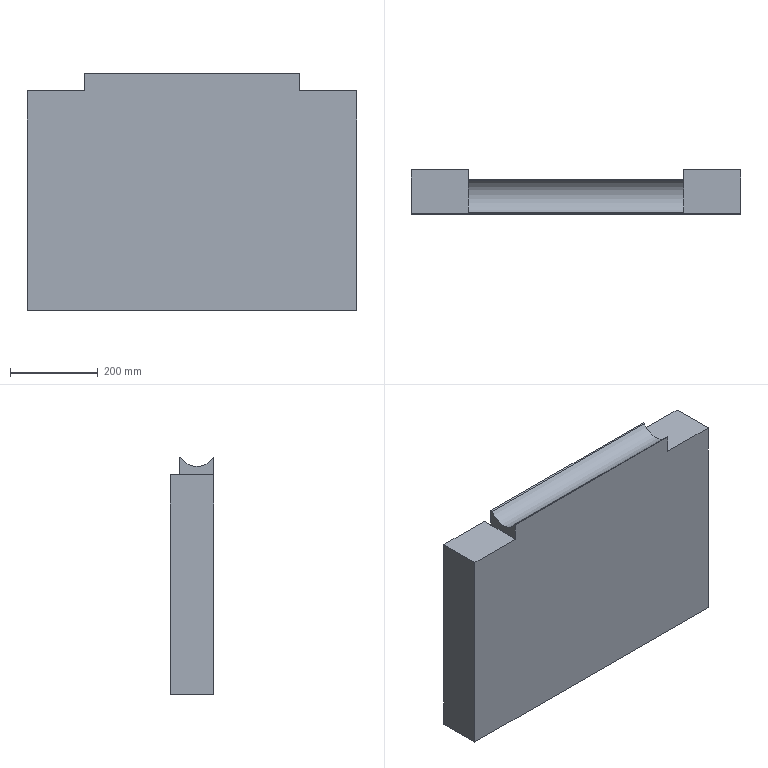Part | STEP file | 1 solid | 16 faces | box 750 x 100 x 540 mm | volume 33368808 mm3 | plane 15 | cylinder 1 | commonest cylinder face diameters 85 x1
STEP:
#1=CARTESIAN_POINT('',(0.,0.,0.));
#2=DIRECTION('',(0.,0.,1.));
#3=DIRECTION('',(1.,0.,0.));
#4=AXIS2_PLACEMENT_3D('',#1,#2,#3);
#5=CARTESIAN_POINT('',(375.,-50.,500.));
#6=VERTEX_POINT('',#5);
#7=CARTESIAN_POINT('',(375.,-50.,0.));
#8=VERTEX_POINT('',#7);
#9=CARTESIAN_POINT('',(375.,-50.,500.));
#10=DIRECTION('',(0.,0.,-1.));
#11=VECTOR('',#10,1.);
#12=LINE('',#9,#11);
#13=CARTESIAN_POINT('',(-375.,-50.,500.));
#14=DIRECTION('',(0.,1.,0.));
#15=DIRECTION('',(0.,0.,1.));
#16=AXIS2_PLACEMENT_3D('',#13,#14,#15);
#17=PLANE('',#16);
#18=CARTESIAN_POINT('',(0.,750.));
#19=DIRECTION('',(-1.,0.));
#20=VECTOR('',#19,1.);
#21=LINE('',#18,#20);
#22=(GEOMETRIC_REPRESENTATION_CONTEXT(2)PARAMETRIC_REPRESENTATION_CONTEXT()REPRESENTATION_CONTEXT('',''));
#23=DEFINITIONAL_REPRESENTATION('',(#21),#22);
#24=PCURVE('',#17,#23);
#25=CARTESIAN_POINT('',(375.,50.,500.));
#26=DIRECTION('',(-1.,0.,0.));
#27=DIRECTION('',(0.,0.,1.));
#28=AXIS2_PLACEMENT_3D('',#25,#26,#27);
#29=PLANE('',#28);
#30=CARTESIAN_POINT('',(0.,-100.));
#31=DIRECTION('',(-1.,0.));
#32=VECTOR('',#31,1.);
#33=LINE('',#30,#32);
#34=(GEOMETRIC_REPRESENTATION_CONTEXT(2)PARAMETRIC_REPRESENTATION_CONTEXT()REPRESENTATION_CONTEXT('',''));
#35=DEFINITIONAL_REPRESENTATION('',(#33),#34);
#36=PCURVE('',#29,#35);
#37=SURFACE_CURVE('',#12,(#24,#36),.PCURVE_S1.);
#38=EDGE_CURVE('',#6,#8,#37,.T.);
#39=ORIENTED_EDGE('',*,*,#38,.F.);
#40=CARTESIAN_POINT('',(245.,-50.,500.));
#41=VERTEX_POINT('',#40);
#42=CARTESIAN_POINT('',(-375.,-50.,500.));
#43=DIRECTION('',(1.,0.,0.));
#44=VECTOR('',#43,1.);
#45=LINE('',#42,#44);
#46=CARTESIAN_POINT('',(0.,0.));
#47=DIRECTION('',(0.,1.));
#48=VECTOR('',#47,1.);
#49=LINE('',#46,#48);
#50=(GEOMETRIC_REPRESENTATION_CONTEXT(2)PARAMETRIC_REPRESENTATION_CONTEXT()REPRESENTATION_CONTEXT('',''));
#51=DEFINITIONAL_REPRESENTATION('',(#49),#50);
#52=PCURVE('',#17,#51);
#53=CARTESIAN_POINT('',(0.,0.,500.));
#54=DIRECTION('',(0.,0.,1.));
#55=DIRECTION('',(1.,0.,0.));
#56=AXIS2_PLACEMENT_3D('',#53,#54,#55);
#57=PLANE('',#56);
#58=CARTESIAN_POINT('',(-375.,-50.));
#59=DIRECTION('',(1.,0.));
#60=VECTOR('',#59,1.);
#61=LINE('',#58,#60);
#62=(GEOMETRIC_REPRESENTATION_CONTEXT(2)PARAMETRIC_REPRESENTATION_CONTEXT()REPRESENTATION_CONTEXT('',''));
#63=DEFINITIONAL_REPRESENTATION('',(#61),#62);
#64=PCURVE('',#57,#63);
#65=SURFACE_CURVE('',#45,(#52,#64),.PCURVE_S1.);
#66=EDGE_CURVE('',#41,#6,#65,.T.);
#67=ORIENTED_EDGE('',*,*,#66,.F.);
#68=CARTESIAN_POINT('',(245.,-50.,540.));
#69=VERTEX_POINT('',#68);
#70=CARTESIAN_POINT('',(245.,-50.,500.));
#71=DIRECTION('',(0.,0.,-1.));
#72=VECTOR('',#71,1.);
#73=LINE('',#70,#72);
#74=CARTESIAN_POINT('',(0.,620.));
#75=DIRECTION('',(-1.,0.));
#76=VECTOR('',#75,1.);
#77=LINE('',#74,#76);
#78=(GEOMETRIC_REPRESENTATION_CONTEXT(2)PARAMETRIC_REPRESENTATION_CONTEXT()REPRESENTATION_CONTEXT('',''));
#79=DEFINITIONAL_REPRESENTATION('',(#77),#78);
#80=PCURVE('',#17,#79);
#81=CARTESIAN_POINT('',(245.,29.,540.));
#82=DIRECTION('',(-1.,0.,0.));
#83=DIRECTION('',(0.,0.,1.));
#84=AXIS2_PLACEMENT_3D('',#81,#82,#83);
#85=PLANE('',#84);
#86=CARTESIAN_POINT('',(-40.,-79.));
#87=DIRECTION('',(-1.,0.));
#88=VECTOR('',#87,1.);
#89=LINE('',#86,#88);
#90=(GEOMETRIC_REPRESENTATION_CONTEXT(2)PARAMETRIC_REPRESENTATION_CONTEXT()REPRESENTATION_CONTEXT('',''));
#91=DEFINITIONAL_REPRESENTATION('',(#89),#90);
#92=PCURVE('',#85,#91);
#93=SURFACE_CURVE('',#73,(#80,#92),.PCURVE_S1.);
#94=EDGE_CURVE('',#69,#41,#93,.T.);
#95=ORIENTED_EDGE('',*,*,#94,.F.);
#96=CARTESIAN_POINT('',(-245.,-50.,540.));
#97=VERTEX_POINT('',#96);
#98=CARTESIAN_POINT('',(-375.,-50.,540.));
#99=DIRECTION('',(1.,0.,0.));
#100=VECTOR('',#99,1.);
#101=LINE('',#98,#100);
#102=CARTESIAN_POINT('',(40.,0.));
#103=DIRECTION('',(0.,1.));
#104=VECTOR('',#103,1.);
#105=LINE('',#102,#104);
#106=(GEOMETRIC_REPRESENTATION_CONTEXT(2)PARAMETRIC_REPRESENTATION_CONTEXT()REPRESENTATION_CONTEXT('',''));
#107=DEFINITIONAL_REPRESENTATION('',(#105),#106);
#108=PCURVE('',#17,#107);
#109=CARTESIAN_POINT('',(0.,0.,540.));
#110=DIRECTION('',(0.,0.,1.));
#111=DIRECTION('',(1.,0.,0.));
#112=AXIS2_PLACEMENT_3D('',#109,#110,#111);
#113=PLANE('',#112);
#114=CARTESIAN_POINT('',(-375.,-50.));
#115=DIRECTION('',(1.,0.));
#116=VECTOR('',#115,1.);
#117=LINE('',#114,#116);
#118=(GEOMETRIC_REPRESENTATION_CONTEXT(2)PARAMETRIC_REPRESENTATION_CONTEXT()REPRESENTATION_CONTEXT('',''));
#119=DEFINITIONAL_REPRESENTATION('',(#117),#118);
#120=PCURVE('',#113,#119);
#121=SURFACE_CURVE('',#101,(#108,#120),.PCURVE_S1.);
#122=EDGE_CURVE('',#97,#69,#121,.T.);
#123=ORIENTED_EDGE('',*,*,#122,.F.);
#124=CARTESIAN_POINT('',(-245.,-50.,500.));
#125=VERTEX_POINT('',#124);
#126=CARTESIAN_POINT('',(-245.,-50.,500.));
#127=DIRECTION('',(0.,0.,1.));
#128=VECTOR('',#127,1.);
#129=LINE('',#126,#128);
#130=CARTESIAN_POINT('',(0.,130.));
#131=DIRECTION('',(1.,0.));
#132=VECTOR('',#131,1.);
#133=LINE('',#130,#132);
#134=(GEOMETRIC_REPRESENTATION_CONTEXT(2)PARAMETRIC_REPRESENTATION_CONTEXT()REPRESENTATION_CONTEXT('',''));
#135=DEFINITIONAL_REPRESENTATION('',(#133),#134);
#136=PCURVE('',#17,#135);
#137=CARTESIAN_POINT('',(-245.,29.,540.));
#138=DIRECTION('',(1.,0.,0.));
#139=DIRECTION('',(0.,0.,-1.));
#140=AXIS2_PLACEMENT_3D('',#137,#138,#139);
#141=PLANE('',#140);
#142=CARTESIAN_POINT('',(40.,-79.));
#143=DIRECTION('',(-1.,0.));
#144=VECTOR('',#143,1.);
#145=LINE('',#142,#144);
#146=(GEOMETRIC_REPRESENTATION_CONTEXT(2)PARAMETRIC_REPRESENTATION_CONTEXT()REPRESENTATION_CONTEXT('',''));
#147=DEFINITIONAL_REPRESENTATION('',(#145),#146);
#148=PCURVE('',#141,#147);
#149=SURFACE_CURVE('',#129,(#136,#148),.PCURVE_S1.);
#150=EDGE_CURVE('',#125,#97,#149,.T.);
#151=ORIENTED_EDGE('',*,*,#150,.F.);
#152=CARTESIAN_POINT('',(-375.,-50.,500.));
#153=VERTEX_POINT('',#152);
#154=CARTESIAN_POINT('',(-375.,-50.,500.));
#155=DIRECTION('',(1.,0.,0.));
#156=VECTOR('',#155,1.);
#157=LINE('',#154,#156);
#158=CARTESIAN_POINT('',(0.,0.));
#159=DIRECTION('',(0.,1.));
#160=VECTOR('',#159,1.);
#161=LINE('',#158,#160);
#162=(GEOMETRIC_REPRESENTATION_CONTEXT(2)PARAMETRIC_REPRESENTATION_CONTEXT()REPRESENTATION_CONTEXT('',''));
#163=DEFINITIONAL_REPRESENTATION('',(#161),#162);
#164=PCURVE('',#17,#163);
#165=CARTESIAN_POINT('',(0.,0.,500.));
#166=DIRECTION('',(0.,0.,1.));
#167=DIRECTION('',(1.,0.,0.));
#168=AXIS2_PLACEMENT_3D('',#165,#166,#167);
#169=PLANE('',#168);
#170=CARTESIAN_POINT('',(-375.,-50.));
#171=DIRECTION('',(1.,0.));
#172=VECTOR('',#171,1.);
#173=LINE('',#170,#172);
#174=(GEOMETRIC_REPRESENTATION_CONTEXT(2)PARAMETRIC_REPRESENTATION_CONTEXT()REPRESENTATION_CONTEXT('',''));
#175=DEFINITIONAL_REPRESENTATION('',(#173),#174);
#176=PCURVE('',#169,#175);
#177=SURFACE_CURVE('',#157,(#164,#176),.PCURVE_S1.);
#178=EDGE_CURVE('',#153,#125,#177,.T.);
#179=ORIENTED_EDGE('',*,*,#178,.F.);
#180=CARTESIAN_POINT('',(-375.,-50.,0.));
#181=VERTEX_POINT('',#180);
#182=CARTESIAN_POINT('',(-375.,-50.,500.));
#183=DIRECTION('',(0.,0.,1.));
#184=VECTOR('',#183,1.);
#185=LINE('',#182,#184);
#186=CARTESIAN_POINT('',(0.,0.));
#187=DIRECTION('',(1.,0.));
#188=VECTOR('',#187,1.);
#189=LINE('',#186,#188);
#190=(GEOMETRIC_REPRESENTATION_CONTEXT(2)PARAMETRIC_REPRESENTATION_CONTEXT()REPRESENTATION_CONTEXT('',''));
#191=DEFINITIONAL_REPRESENTATION('',(#189),#190);
#192=PCURVE('',#17,#191);
#193=CARTESIAN_POINT('',(-375.,50.,500.));
#194=DIRECTION('',(1.,0.,0.));
#195=DIRECTION('',(0.,0.,-1.));
#196=AXIS2_PLACEMENT_3D('',#193,#194,#195);
#197=PLANE('',#196);
#198=CARTESIAN_POINT('',(0.,-100.));
#199=DIRECTION('',(-1.,0.));
#200=VECTOR('',#199,1.);
#201=LINE('',#198,#200);
#202=(GEOMETRIC_REPRESENTATION_CONTEXT(2)PARAMETRIC_REPRESENTATION_CONTEXT()REPRESENTATION_CONTEXT('',''));
#203=DEFINITIONAL_REPRESENTATION('',(#201),#202);
#204=PCURVE('',#197,#203);
#205=SURFACE_CURVE('',#185,(#192,#204),.PCURVE_S1.);
#206=EDGE_CURVE('',#181,#153,#205,.T.);
#207=ORIENTED_EDGE('',*,*,#206,.F.);
#208=CARTESIAN_POINT('',(-375.,-50.,0.));
#209=DIRECTION('',(-1.,0.,0.));
#210=VECTOR('',#209,1.);
#211=LINE('',#208,#210);
#212=CARTESIAN_POINT('',(-500.,0.));
#213=DIRECTION('',(0.,-1.));
#214=VECTOR('',#213,1.);
#215=LINE('',#212,#214);
#216=(GEOMETRIC_REPRESENTATION_CONTEXT(2)PARAMETRIC_REPRESENTATION_CONTEXT()REPRESENTATION_CONTEXT('',''));
#217=DEFINITIONAL_REPRESENTATION('',(#215),#216);
#218=PCURVE('',#17,#217);
#219=CARTESIAN_POINT('',(0.,0.,0.));
#220=DIRECTION('',(0.,0.,1.));
#221=DIRECTION('',(1.,0.,0.));
#222=AXIS2_PLACEMENT_3D('',#219,#220,#221);
#223=PLANE('',#222);
#224=CARTESIAN_POINT('',(-375.,-50.));
#225=DIRECTION('',(-1.,0.));
#226=VECTOR('',#225,1.);
#227=LINE('',#224,#226);
#228=(GEOMETRIC_REPRESENTATION_CONTEXT(2)PARAMETRIC_REPRESENTATION_CONTEXT()REPRESENTATION_CONTEXT('',''));
#229=DEFINITIONAL_REPRESENTATION('',(#227),#228);
#230=PCURVE('',#223,#229);
#231=SURFACE_CURVE('',#211,(#218,#230),.PCURVE_S1.);
#232=EDGE_CURVE('',#8,#181,#231,.T.);
#233=ORIENTED_EDGE('',*,*,#232,.F.);
#234=EDGE_LOOP('',(#39,#67,#95,#123,#151,#179,#207,#233));
#235=FACE_BOUND('',#234,.T.);
#236=ADVANCED_FACE('',(#235),#17,.F.);
#237=CARTESIAN_POINT('',(245.,50.,0.));
#238=VERTEX_POINT('',#237);
#239=CARTESIAN_POINT('',(245.,29.,0.));
#240=VERTEX_POINT('',#239);
#241=CARTESIAN_POINT('',(245.,0.,0.));
#242=DIRECTION('',(0.,-1.,0.));
#243=VECTOR('',#242,1.);
#244=LINE('',#241,#243);
#245=CARTESIAN_POINT('',(245.,0.));
#246=DIRECTION('',(0.,-1.));
#247=VECTOR('',#246,1.);
#248=LINE('',#245,#247);
#249=(GEOMETRIC_REPRESENTATION_CONTEXT(2)PARAMETRIC_REPRESENTATION_CONTEXT()REPRESENTATION_CONTEXT('',''));
#250=DEFINITIONAL_REPRESENTATION('',(#248),#249);
#251=PCURVE('',#223,#250);
#252=CARTESIAN_POINT('',(245.,71.,0.));
#253=DIRECTION('',(1.,0.,0.));
#254=DIRECTION('',(0.,0.,-1.));
#255=AXIS2_PLACEMENT_3D('',#252,#253,#254);
#256=PLANE('',#255);
#257=CARTESIAN_POINT('',(0.,-71.));
#258=DIRECTION('',(0.,-1.));
#259=VECTOR('',#258,1.);
#260=LINE('',#257,#259);
#261=(GEOMETRIC_REPRESENTATION_CONTEXT(2)PARAMETRIC_REPRESENTATION_CONTEXT()REPRESENTATION_CONTEXT('',''));
#262=DEFINITIONAL_REPRESENTATION('',(#260),#261);
#263=PCURVE('',#256,#262);
#264=SURFACE_CURVE('',#244,(#251,#263),.PCURVE_S1.);
#265=EDGE_CURVE('',#238,#240,#264,.T.);
#266=ORIENTED_EDGE('',*,*,#265,.F.);
#267=CARTESIAN_POINT('',(375.,50.,0.));
#268=VERTEX_POINT('',#267);
#269=CARTESIAN_POINT('',(0.,50.,0.));
#270=DIRECTION('',(-1.,0.,0.));
#271=VECTOR('',#270,1.);
#272=LINE('',#269,#271);
#273=CARTESIAN_POINT('',(0.,50.));
#274=DIRECTION('',(-1.,0.));
#275=VECTOR('',#274,1.);
#276=LINE('',#273,#275);
#277=(GEOMETRIC_REPRESENTATION_CONTEXT(2)PARAMETRIC_REPRESENTATION_CONTEXT()REPRESENTATION_CONTEXT('',''));
#278=DEFINITIONAL_REPRESENTATION('',(#276),#277);
#279=PCURVE('',#223,#278);
#280=CARTESIAN_POINT('',(-375.,50.,500.));
#281=DIRECTION('',(0.,-1.,0.));
#282=DIRECTION('',(0.,0.,-1.));
#283=AXIS2_PLACEMENT_3D('',#280,#281,#282);
#284=PLANE('',#283);
#285=CARTESIAN_POINT('',(500.,375.));
#286=DIRECTION('',(0.,-1.));
#287=VECTOR('',#286,1.);
#288=LINE('',#285,#287);
#289=(GEOMETRIC_REPRESENTATION_CONTEXT(2)PARAMETRIC_REPRESENTATION_CONTEXT()REPRESENTATION_CONTEXT('',''));
#290=DEFINITIONAL_REPRESENTATION('',(#288),#289);
#291=PCURVE('',#284,#290);
#292=SURFACE_CURVE('',#272,(#279,#291),.PCURVE_S1.);
#293=EDGE_CURVE('',#268,#238,#292,.T.);
#294=ORIENTED_EDGE('',*,*,#293,.F.);
#295=CARTESIAN_POINT('',(375.,0.,0.));
#296=DIRECTION('',(0.,1.,0.));
#297=VECTOR('',#296,1.);
#298=LINE('',#295,#297);
#299=CARTESIAN_POINT('',(375.,0.));
#300=DIRECTION('',(0.,1.));
#301=VECTOR('',#300,1.);
#302=LINE('',#299,#301);
#303=(GEOMETRIC_REPRESENTATION_CONTEXT(2)PARAMETRIC_REPRESENTATION_CONTEXT()REPRESENTATION_CONTEXT('',''));
#304=DEFINITIONAL_REPRESENTATION('',(#302),#303);
#305=PCURVE('',#223,#304);
#306=CARTESIAN_POINT('',(-500.,-50.));
#307=DIRECTION('',(0.,1.));
#308=VECTOR('',#307,1.);
#309=LINE('',#306,#308);
#310=(GEOMETRIC_REPRESENTATION_CONTEXT(2)PARAMETRIC_REPRESENTATION_CONTEXT()REPRESENTATION_CONTEXT('',''));
#311=DEFINITIONAL_REPRESENTATION('',(#309),#310);
#312=PCURVE('',#29,#311);
#313=SURFACE_CURVE('',#298,(#305,#312),.PCURVE_S1.);
#314=EDGE_CURVE('',#8,#268,#313,.T.);
#315=ORIENTED_EDGE('',*,*,#314,.F.);
#316=ORIENTED_EDGE('',*,*,#232,.T.);
#317=CARTESIAN_POINT('',(-375.,50.,0.));
#318=VERTEX_POINT('',#317);
#319=CARTESIAN_POINT('',(-375.,0.,0.));
#320=DIRECTION('',(0.,-1.,0.));
#321=VECTOR('',#320,1.);
#322=LINE('',#319,#321);
#323=CARTESIAN_POINT('',(-375.,0.));
#324=DIRECTION('',(0.,-1.));
#325=VECTOR('',#324,1.);
#326=LINE('',#323,#325);
#327=(GEOMETRIC_REPRESENTATION_CONTEXT(2)PARAMETRIC_REPRESENTATION_CONTEXT()REPRESENTATION_CONTEXT('',''));
#328=DEFINITIONAL_REPRESENTATION('',(#326),#327);
#329=PCURVE('',#223,#328);
#330=CARTESIAN_POINT('',(500.,-50.));
#331=DIRECTION('',(0.,-1.));
#332=VECTOR('',#331,1.);
#333=LINE('',#330,#332);
#334=(GEOMETRIC_REPRESENTATION_CONTEXT(2)PARAMETRIC_REPRESENTATION_CONTEXT()REPRESENTATION_CONTEXT('',''));
#335=DEFINITIONAL_REPRESENTATION('',(#333),#334);
#336=PCURVE('',#197,#335);
#337=SURFACE_CURVE('',#322,(#329,#336),.PCURVE_S1.);
#338=EDGE_CURVE('',#318,#181,#337,.T.);
#339=ORIENTED_EDGE('',*,*,#338,.F.);
#340=CARTESIAN_POINT('',(-245.,50.,0.));
#341=VERTEX_POINT('',#340);
#342=CARTESIAN_POINT('',(0.,50.,0.));
#343=DIRECTION('',(-1.,0.,0.));
#344=VECTOR('',#343,1.);
#345=LINE('',#342,#344);
#346=CARTESIAN_POINT('',(0.,50.));
#347=DIRECTION('',(-1.,0.));
#348=VECTOR('',#347,1.);
#349=LINE('',#346,#348);
#350=(GEOMETRIC_REPRESENTATION_CONTEXT(2)PARAMETRIC_REPRESENTATION_CONTEXT()REPRESENTATION_CONTEXT('',''));
#351=DEFINITIONAL_REPRESENTATION('',(#349),#350);
#352=PCURVE('',#223,#351);
#353=CARTESIAN_POINT('',(-375.,50.,500.));
#354=DIRECTION('',(0.,-1.,0.));
#355=DIRECTION('',(0.,0.,-1.));
#356=AXIS2_PLACEMENT_3D('',#353,#354,#355);
#357=PLANE('',#356);
#358=CARTESIAN_POINT('',(500.,375.));
#359=DIRECTION('',(0.,-1.));
#360=VECTOR('',#359,1.);
#361=LINE('',#358,#360);
#362=(GEOMETRIC_REPRESENTATION_CONTEXT(2)PARAMETRIC_REPRESENTATION_CONTEXT()REPRESENTATION_CONTEXT('',''));
#363=DEFINITIONAL_REPRESENTATION('',(#361),#362);
#364=PCURVE('',#357,#363);
#365=SURFACE_CURVE('',#345,(#352,#364),.PCURVE_S1.);
#366=EDGE_CURVE('',#341,#318,#365,.T.);
#367=ORIENTED_EDGE('',*,*,#366,.F.);
#368=CARTESIAN_POINT('',(-245.,29.,0.));
#369=VERTEX_POINT('',#368);
#370=CARTESIAN_POINT('',(-245.,0.,0.));
#371=DIRECTION('',(0.,1.,0.));
#372=VECTOR('',#371,1.);
#373=LINE('',#370,#372);
#374=CARTESIAN_POINT('',(-245.,0.));
#375=DIRECTION('',(0.,1.));
#376=VECTOR('',#375,1.);
#377=LINE('',#374,#376);
#378=(GEOMETRIC_REPRESENTATION_CONTEXT(2)PARAMETRIC_REPRESENTATION_CONTEXT()REPRESENTATION_CONTEXT('',''));
#379=DEFINITIONAL_REPRESENTATION('',(#377),#378);
#380=PCURVE('',#223,#379);
#381=CARTESIAN_POINT('',(-245.,71.,0.));
#382=DIRECTION('',(-1.,0.,0.));
#383=DIRECTION('',(0.,0.,1.));
#384=AXIS2_PLACEMENT_3D('',#381,#382,#383);
#385=PLANE('',#384);
#386=CARTESIAN_POINT('',(0.,-71.));
#387=DIRECTION('',(0.,1.));
#388=VECTOR('',#387,1.);
#389=LINE('',#386,#388);
#390=(GEOMETRIC_REPRESENTATION_CONTEXT(2)PARAMETRIC_REPRESENTATION_CONTEXT()REPRESENTATION_CONTEXT('',''));
#391=DEFINITIONAL_REPRESENTATION('',(#389),#390);
#392=PCURVE('',#385,#391);
#393=SURFACE_CURVE('',#373,(#380,#392),.PCURVE_S1.);
#394=EDGE_CURVE('',#369,#341,#393,.T.);
#395=ORIENTED_EDGE('',*,*,#394,.F.);
#396=CARTESIAN_POINT('',(0.,29.,0.));
#397=DIRECTION('',(-1.,0.,0.));
#398=VECTOR('',#397,1.);
#399=LINE('',#396,#398);
#400=CARTESIAN_POINT('',(0.,29.));
#401=DIRECTION('',(-1.,0.));
#402=VECTOR('',#401,1.);
#403=LINE('',#400,#402);
#404=(GEOMETRIC_REPRESENTATION_CONTEXT(2)PARAMETRIC_REPRESENTATION_CONTEXT()REPRESENTATION_CONTEXT('',''));
#405=DEFINITIONAL_REPRESENTATION('',(#403),#404);
#406=PCURVE('',#223,#405);
#407=CARTESIAN_POINT('',(-245.,29.,0.));
#408=DIRECTION('',(0.,-1.,0.));
#409=DIRECTION('',(0.,0.,-1.));
#410=AXIS2_PLACEMENT_3D('',#407,#408,#409);
#411=PLANE('',#410);
#412=CARTESIAN_POINT('',(0.,245.));
#413=DIRECTION('',(0.,-1.));
#414=VECTOR('',#413,1.);
#415=LINE('',#412,#414);
#416=(GEOMETRIC_REPRESENTATION_CONTEXT(2)PARAMETRIC_REPRESENTATION_CONTEXT()REPRESENTATION_CONTEXT('',''));
#417=DEFINITIONAL_REPRESENTATION('',(#415),#416);
#418=PCURVE('',#411,#417);
#419=SURFACE_CURVE('',#399,(#406,#418),.PCURVE_S1.);
#420=EDGE_CURVE('',#240,#369,#419,.T.);
#421=ORIENTED_EDGE('',*,*,#420,.F.);
#422=EDGE_LOOP('',(#266,#294,#315,#316,#339,#367,#395,#421));
#423=FACE_BOUND('',#422,.T.);
#424=ADVANCED_FACE('',(#423),#223,.F.);
#425=CARTESIAN_POINT('',(375.,50.,500.));
#426=VERTEX_POINT('',#425);
#427=CARTESIAN_POINT('',(375.,50.,500.));
#428=DIRECTION('',(0.,0.,-1.));
#429=VECTOR('',#428,1.);
#430=LINE('',#427,#429);
#431=CARTESIAN_POINT('',(0.,0.));
#432=DIRECTION('',(-1.,0.));
#433=VECTOR('',#432,1.);
#434=LINE('',#431,#433);
#435=(GEOMETRIC_REPRESENTATION_CONTEXT(2)PARAMETRIC_REPRESENTATION_CONTEXT()REPRESENTATION_CONTEXT('',''));
#436=DEFINITIONAL_REPRESENTATION('',(#434),#435);
#437=PCURVE('',#29,#436);
#438=CARTESIAN_POINT('',(0.,750.));
#439=DIRECTION('',(1.,0.));
#440=VECTOR('',#439,1.);
#441=LINE('',#438,#440);
#442=(GEOMETRIC_REPRESENTATION_CONTEXT(2)PARAMETRIC_REPRESENTATION_CONTEXT()REPRESENTATION_CONTEXT('',''));
#443=DEFINITIONAL_REPRESENTATION('',(#441),#442);
#444=PCURVE('',#284,#443);
#445=SURFACE_CURVE('',#430,(#437,#444),.PCURVE_S1.);
#446=EDGE_CURVE('',#426,#268,#445,.T.);
#447=ORIENTED_EDGE('',*,*,#446,.F.);
#448=CARTESIAN_POINT('',(375.,50.,500.));
#449=DIRECTION('',(0.,1.,0.));
#450=VECTOR('',#449,1.);
#451=LINE('',#448,#450);
#452=CARTESIAN_POINT('',(0.,0.));
#453=DIRECTION('',(0.,1.));
#454=VECTOR('',#453,1.);
#455=LINE('',#452,#454);
#456=(GEOMETRIC_REPRESENTATION_CONTEXT(2)PARAMETRIC_REPRESENTATION_CONTEXT()REPRESENTATION_CONTEXT('',''));
#457=DEFINITIONAL_REPRESENTATION('',(#455),#456);
#458=PCURVE('',#29,#457);
#459=CARTESIAN_POINT('',(375.,50.));
#460=DIRECTION('',(0.,1.));
#461=VECTOR('',#460,1.);
#462=LINE('',#459,#461);
#463=(GEOMETRIC_REPRESENTATION_CONTEXT(2)PARAMETRIC_REPRESENTATION_CONTEXT()REPRESENTATION_CONTEXT('',''));
#464=DEFINITIONAL_REPRESENTATION('',(#462),#463);
#465=PCURVE('',#57,#464);
#466=SURFACE_CURVE('',#451,(#458,#465),.PCURVE_S1.);
#467=EDGE_CURVE('',#6,#426,#466,.T.);
#468=ORIENTED_EDGE('',*,*,#467,.F.);
#469=ORIENTED_EDGE('',*,*,#38,.T.);
#470=ORIENTED_EDGE('',*,*,#314,.T.);
#471=EDGE_LOOP('',(#447,#468,#469,#470));
#472=FACE_BOUND('',#471,.T.);
#473=ADVANCED_FACE('',(#472),#29,.F.);
#474=CARTESIAN_POINT('',(245.,50.,500.));
#475=VERTEX_POINT('',#474);
#476=CARTESIAN_POINT('',(0.,50.,500.));
#477=DIRECTION('',(-1.,0.,0.));
#478=VECTOR('',#477,1.);
#479=LINE('',#476,#478);
#480=CARTESIAN_POINT('',(0.,50.));
#481=DIRECTION('',(-1.,0.));
#482=VECTOR('',#481,1.);
#483=LINE('',#480,#482);
#484=(GEOMETRIC_REPRESENTATION_CONTEXT(2)PARAMETRIC_REPRESENTATION_CONTEXT()REPRESENTATION_CONTEXT('',''));
#485=DEFINITIONAL_REPRESENTATION('',(#483),#484);
#486=PCURVE('',#57,#485);
#487=CARTESIAN_POINT('',(0.,375.));
#488=DIRECTION('',(0.,-1.));
#489=VECTOR('',#488,1.);
#490=LINE('',#487,#489);
#491=(GEOMETRIC_REPRESENTATION_CONTEXT(2)PARAMETRIC_REPRESENTATION_CONTEXT()REPRESENTATION_CONTEXT('',''));
#492=DEFINITIONAL_REPRESENTATION('',(#490),#491);
#493=PCURVE('',#284,#492);
#494=SURFACE_CURVE('',#479,(#486,#493),.PCURVE_S1.);
#495=EDGE_CURVE('',#426,#475,#494,.T.);
#496=ORIENTED_EDGE('',*,*,#495,.T.);
#497=CARTESIAN_POINT('',(245.,29.,500.));
#498=VERTEX_POINT('',#497);
#499=CARTESIAN_POINT('',(245.,0.,500.));
#500=DIRECTION('',(0.,-1.,0.));
#501=VECTOR('',#500,1.);
#502=LINE('',#499,#501);
#503=CARTESIAN_POINT('',(245.,0.));
#504=DIRECTION('',(0.,-1.));
#505=VECTOR('',#504,1.);
#506=LINE('',#503,#505);
#507=(GEOMETRIC_REPRESENTATION_CONTEXT(2)PARAMETRIC_REPRESENTATION_CONTEXT()REPRESENTATION_CONTEXT('',''));
#508=DEFINITIONAL_REPRESENTATION('',(#506),#507);
#509=PCURVE('',#57,#508);
#510=CARTESIAN_POINT('',(-500.,-71.));
#511=DIRECTION('',(0.,-1.));
#512=VECTOR('',#511,1.);
#513=LINE('',#510,#512);
#514=(GEOMETRIC_REPRESENTATION_CONTEXT(2)PARAMETRIC_REPRESENTATION_CONTEXT()REPRESENTATION_CONTEXT('',''));
#515=DEFINITIONAL_REPRESENTATION('',(#513),#514);
#516=PCURVE('',#256,#515);
#517=SURFACE_CURVE('',#502,(#509,#516),.PCURVE_S1.);
#518=EDGE_CURVE('',#475,#498,#517,.T.);
#519=ORIENTED_EDGE('',*,*,#518,.T.);
#520=CARTESIAN_POINT('',(245.,0.,500.));
#521=DIRECTION('',(0.,-1.,0.));
#522=VECTOR('',#521,1.);
#523=LINE('',#520,#522);
#524=CARTESIAN_POINT('',(245.,0.));
#525=DIRECTION('',(0.,-1.));
#526=VECTOR('',#525,1.);
#527=LINE('',#524,#526);
#528=(GEOMETRIC_REPRESENTATION_CONTEXT(2)PARAMETRIC_REPRESENTATION_CONTEXT()REPRESENTATION_CONTEXT('',''));
#529=DEFINITIONAL_REPRESENTATION('',(#527),#528);
#530=PCURVE('',#57,#529);
#531=CARTESIAN_POINT('',(-40.,-29.));
#532=DIRECTION('',(0.,-1.));
#533=VECTOR('',#532,1.);
#534=LINE('',#531,#533);
#535=(GEOMETRIC_REPRESENTATION_CONTEXT(2)PARAMETRIC_REPRESENTATION_CONTEXT()REPRESENTATION_CONTEXT('',''));
#536=DEFINITIONAL_REPRESENTATION('',(#534),#535);
#537=PCURVE('',#85,#536);
#538=SURFACE_CURVE('',#523,(#530,#537),.PCURVE_S1.);
#539=EDGE_CURVE('',#498,#41,#538,.T.);
#540=ORIENTED_EDGE('',*,*,#539,.T.);
#541=ORIENTED_EDGE('',*,*,#66,.T.);
#542=ORIENTED_EDGE('',*,*,#467,.T.);
#543=EDGE_LOOP('',(#496,#519,#540,#541,#542));
#544=FACE_BOUND('',#543,.T.);
#545=ADVANCED_FACE('',(#544),#57,.T.);
#546=CARTESIAN_POINT('',(245.,-48.161,540.));
#547=VERTEX_POINT('',#546);
#548=CARTESIAN_POINT('',(245.,25.161,540.));
#549=VERTEX_POINT('',#548);
#550=CARTESIAN_POINT('',(245.,-11.5,561.5));
#551=DIRECTION('',(1.,0.,0.));
#552=DIRECTION('',(0.,0.,1.));
#553=AXIS2_PLACEMENT_3D('',#550,#551,#552);
#554=CIRCLE('',#553,42.5);
#555=CARTESIAN_POINT('',(64.,-40.5));
#556=CARTESIAN_POINT('',(64.,-114.112));
#557=CARTESIAN_POINT('',(0.25,-77.306));
#558=CARTESIAN_POINT('',(-63.5,-40.5));
#559=CARTESIAN_POINT('',(0.25,-3.694));
#560=CARTESIAN_POINT('',(64.,33.112));
#561=CARTESIAN_POINT('',(64.,-40.5));
#562=(BOUNDED_CURVE()B_SPLINE_CURVE(2,(#555,#556,#557,#558,#559,#560,#561),.UNSPECIFIED.,.T.,.F.)B_SPLINE_CURVE_WITH_KNOTS((1,2,2,2,2,1),(-2.094,0.,2.094,4.189,6.283,8.378),.UNSPECIFIED.)CURVE()GEOMETRIC_REPRESENTATION_ITEM()RATIONAL_B_SPLINE_CURVE((1.,0.5,1.,0.5,1.,0.5,1.))REPRESENTATION_ITEM(''));
#563=(GEOMETRIC_REPRESENTATION_CONTEXT(2)PARAMETRIC_REPRESENTATION_CONTEXT()REPRESENTATION_CONTEXT('',''));
#564=DEFINITIONAL_REPRESENTATION('',(#562),#563);
#565=PCURVE('',#85,#564);
#566=CARTESIAN_POINT('',(-303.,-11.5,561.5));
#567=DIRECTION('',(-1.,0.,0.));
#568=DIRECTION('',(0.,0.,1.));
#569=AXIS2_PLACEMENT_3D('',#566,#567,#568);
#570=CYLINDRICAL_SURFACE('',#569,42.5);
#571=CARTESIAN_POINT('',(6.283,-548.));
#572=DIRECTION('',(-1.,0.));
#573=VECTOR('',#572,1.);
#574=LINE('',#571,#573);
#575=(GEOMETRIC_REPRESENTATION_CONTEXT(2)PARAMETRIC_REPRESENTATION_CONTEXT()REPRESENTATION_CONTEXT('',''));
#576=DEFINITIONAL_REPRESENTATION('',(#574),#575);
#577=PCURVE('',#570,#576);
#578=SURFACE_CURVE('',#554,(#565,#577),.PCURVE_S1.);
#579=EDGE_CURVE('',#547,#549,#578,.T.);
#580=ORIENTED_EDGE('',*,*,#579,.F.);
#581=CARTESIAN_POINT('',(245.,29.,540.));
#582=DIRECTION('',(0.,1.,0.));
#583=VECTOR('',#582,1.);
#584=LINE('',#581,#583);
#585=CARTESIAN_POINT('',(0.,0.));
#586=DIRECTION('',(0.,1.));
#587=VECTOR('',#586,1.);
#588=LINE('',#585,#587);
#589=(GEOMETRIC_REPRESENTATION_CONTEXT(2)PARAMETRIC_REPRESENTATION_CONTEXT()REPRESENTATION_CONTEXT('',''));
#590=DEFINITIONAL_REPRESENTATION('',(#588),#589);
#591=PCURVE('',#85,#590);
#592=CARTESIAN_POINT('',(245.,29.));
#593=DIRECTION('',(0.,1.));
#594=VECTOR('',#593,1.);
#595=LINE('',#592,#594);
#596=(GEOMETRIC_REPRESENTATION_CONTEXT(2)PARAMETRIC_REPRESENTATION_CONTEXT()REPRESENTATION_CONTEXT('',''));
#597=DEFINITIONAL_REPRESENTATION('',(#595),#596);
#598=PCURVE('',#113,#597);
#599=SURFACE_CURVE('',#584,(#591,#598),.PCURVE_S1.);
#600=EDGE_CURVE('',#69,#547,#599,.T.);
#601=ORIENTED_EDGE('',*,*,#600,.F.);
#602=ORIENTED_EDGE('',*,*,#94,.T.);
#603=ORIENTED_EDGE('',*,*,#539,.F.);
#604=CARTESIAN_POINT('',(245.,29.,540.));
#605=VERTEX_POINT('',#604);
#606=CARTESIAN_POINT('',(245.,29.,540.));
#607=DIRECTION('',(0.,0.,-1.));
#608=VECTOR('',#607,1.);
#609=LINE('',#606,#608);
#610=CARTESIAN_POINT('',(0.,0.));
#611=DIRECTION('',(-1.,0.));
#612=VECTOR('',#611,1.);
#613=LINE('',#610,#612);
#614=(GEOMETRIC_REPRESENTATION_CONTEXT(2)PARAMETRIC_REPRESENTATION_CONTEXT()REPRESENTATION_CONTEXT('',''));
#615=DEFINITIONAL_REPRESENTATION('',(#613),#614);
#616=PCURVE('',#85,#615);
#617=CARTESIAN_POINT('',(-540.,490.));
#618=DIRECTION('',(1.,0.));
#619=VECTOR('',#618,1.);
#620=LINE('',#617,#619);
#621=(GEOMETRIC_REPRESENTATION_CONTEXT(2)PARAMETRIC_REPRESENTATION_CONTEXT()REPRESENTATION_CONTEXT('',''));
#622=DEFINITIONAL_REPRESENTATION('',(#620),#621);
#623=PCURVE('',#411,#622);
#624=SURFACE_CURVE('',#609,(#616,#623),.PCURVE_S1.);
#625=EDGE_CURVE('',#605,#498,#624,.T.);
#626=ORIENTED_EDGE('',*,*,#625,.F.);
#627=CARTESIAN_POINT('',(245.,29.,540.));
#628=DIRECTION('',(0.,1.,0.));
#629=VECTOR('',#628,1.);
#630=LINE('',#627,#629);
#631=CARTESIAN_POINT('',(0.,0.));
#632=DIRECTION('',(0.,1.));
#633=VECTOR('',#632,1.);
#634=LINE('',#631,#633);
#635=(GEOMETRIC_REPRESENTATION_CONTEXT(2)PARAMETRIC_REPRESENTATION_CONTEXT()REPRESENTATION_CONTEXT('',''));
#636=DEFINITIONAL_REPRESENTATION('',(#634),#635);
#637=PCURVE('',#85,#636);
#638=CARTESIAN_POINT('',(0.,0.,540.));
#639=DIRECTION('',(0.,0.,1.));
#640=DIRECTION('',(1.,0.,0.));
#641=AXIS2_PLACEMENT_3D('',#638,#639,#640);
#642=PLANE('',#641);
#643=CARTESIAN_POINT('',(245.,29.));
#644=DIRECTION('',(0.,1.));
#645=VECTOR('',#644,1.);
#646=LINE('',#643,#645);
#647=(GEOMETRIC_REPRESENTATION_CONTEXT(2)PARAMETRIC_REPRESENTATION_CONTEXT()REPRESENTATION_CONTEXT('',''));
#648=DEFINITIONAL_REPRESENTATION('',(#646),#647);
#649=PCURVE('',#642,#648);
#650=SURFACE_CURVE('',#630,(#637,#649),.PCURVE_S1.);
#651=EDGE_CURVE('',#549,#605,#650,.T.);
#652=ORIENTED_EDGE('',*,*,#651,.F.);
#653=EDGE_LOOP('',(#580,#601,#602,#603,#626,#652));
#654=FACE_BOUND('',#653,.T.);
#655=ADVANCED_FACE('',(#654),#85,.F.);
#656=ORIENTED_EDGE('',*,*,#122,.T.);
#657=ORIENTED_EDGE('',*,*,#600,.T.);
#658=CARTESIAN_POINT('',(-245.,-48.161,540.));
#659=VERTEX_POINT('',#658);
#660=CARTESIAN_POINT('',(0.,-48.161,540.));
#661=DIRECTION('',(-1.,0.,0.));
#662=VECTOR('',#661,1.);
#663=LINE('',#660,#662);
#664=CARTESIAN_POINT('',(0.,-48.161));
#665=DIRECTION('',(-1.,0.));
#666=VECTOR('',#665,1.);
#667=LINE('',#664,#666);
#668=(GEOMETRIC_REPRESENTATION_CONTEXT(2)PARAMETRIC_REPRESENTATION_CONTEXT()REPRESENTATION_CONTEXT('',''));
#669=DEFINITIONAL_REPRESENTATION('',(#667),#668);
#670=PCURVE('',#113,#669);
#671=CARTESIAN_POINT('',(4.182,-303.));
#672=DIRECTION('',(0.,1.));
#673=VECTOR('',#672,1.);
#674=LINE('',#671,#673);
#675=(GEOMETRIC_REPRESENTATION_CONTEXT(2)PARAMETRIC_REPRESENTATION_CONTEXT()REPRESENTATION_CONTEXT('',''));
#676=DEFINITIONAL_REPRESENTATION('',(#674),#675);
#677=PCURVE('',#570,#676);
#678=SURFACE_CURVE('',#663,(#670,#677),.PCURVE_S1.);
#679=EDGE_CURVE('',#547,#659,#678,.T.);
#680=ORIENTED_EDGE('',*,*,#679,.T.);
#681=CARTESIAN_POINT('',(-245.,0.,540.));
#682=DIRECTION('',(0.,-1.,0.));
#683=VECTOR('',#682,1.);
#684=LINE('',#681,#683);
#685=CARTESIAN_POINT('',(-245.,0.));
#686=DIRECTION('',(0.,-1.));
#687=VECTOR('',#686,1.);
#688=LINE('',#685,#687);
#689=(GEOMETRIC_REPRESENTATION_CONTEXT(2)PARAMETRIC_REPRESENTATION_CONTEXT()REPRESENTATION_CONTEXT('',''));
#690=DEFINITIONAL_REPRESENTATION('',(#688),#689);
#691=PCURVE('',#113,#690);
#692=CARTESIAN_POINT('',(0.,-29.));
#693=DIRECTION('',(0.,-1.));
#694=VECTOR('',#693,1.);
#695=LINE('',#692,#694);
#696=(GEOMETRIC_REPRESENTATION_CONTEXT(2)PARAMETRIC_REPRESENTATION_CONTEXT()REPRESENTATION_CONTEXT('',''));
#697=DEFINITIONAL_REPRESENTATION('',(#695),#696);
#698=PCURVE('',#141,#697);
#699=SURFACE_CURVE('',#684,(#691,#698),.PCURVE_S1.);
#700=EDGE_CURVE('',#659,#97,#699,.T.);
#701=ORIENTED_EDGE('',*,*,#700,.T.);
#702=EDGE_LOOP('',(#656,#657,#680,#701));
#703=FACE_BOUND('',#702,.T.);
#704=ADVANCED_FACE('',(#703),#113,.T.);
#705=CARTESIAN_POINT('',(-245.,25.161,540.));
#706=VERTEX_POINT('',#705);
#707=CARTESIAN_POINT('',(-245.,-11.5,561.5));
#708=DIRECTION('',(-1.,0.,0.));
#709=DIRECTION('',(0.,0.,1.));
#710=AXIS2_PLACEMENT_3D('',#707,#708,#709);
#711=CIRCLE('',#710,42.5);
#712=CARTESIAN_POINT('',(-64.,-40.5));
#713=CARTESIAN_POINT('',(-64.,33.112));
#714=CARTESIAN_POINT('',(-0.25,-3.694));
#715=CARTESIAN_POINT('',(63.5,-40.5));
#716=CARTESIAN_POINT('',(-0.25,-77.306));
#717=CARTESIAN_POINT('',(-64.,-114.112));
#718=CARTESIAN_POINT('',(-64.,-40.5));
#719=(BOUNDED_CURVE()B_SPLINE_CURVE(2,(#712,#713,#714,#715,#716,#717,#718),.UNSPECIFIED.,.T.,.F.)B_SPLINE_CURVE_WITH_KNOTS((1,2,2,2,2,1),(-2.094,0.,2.094,4.189,6.283,8.378),.UNSPECIFIED.)CURVE()GEOMETRIC_REPRESENTATION_ITEM()RATIONAL_B_SPLINE_CURVE((1.,0.5,1.,0.5,1.,0.5,1.))REPRESENTATION_ITEM(''));
#720=(GEOMETRIC_REPRESENTATION_CONTEXT(2)PARAMETRIC_REPRESENTATION_CONTEXT()REPRESENTATION_CONTEXT('',''));
#721=DEFINITIONAL_REPRESENTATION('',(#719),#720);
#722=PCURVE('',#141,#721);
#723=CARTESIAN_POINT('',(0.,-58.));
#724=DIRECTION('',(1.,0.));
#725=VECTOR('',#724,1.);
#726=LINE('',#723,#725);
#727=(GEOMETRIC_REPRESENTATION_CONTEXT(2)PARAMETRIC_REPRESENTATION_CONTEXT()REPRESENTATION_CONTEXT('',''));
#728=DEFINITIONAL_REPRESENTATION('',(#726),#727);
#729=PCURVE('',#570,#728);
#730=SURFACE_CURVE('',#711,(#722,#729),.PCURVE_S1.);
#731=EDGE_CURVE('',#706,#659,#730,.T.);
#732=ORIENTED_EDGE('',*,*,#731,.F.);
#733=CARTESIAN_POINT('',(-245.,29.,540.));
#734=VERTEX_POINT('',#733);
#735=CARTESIAN_POINT('',(-245.,29.,540.));
#736=DIRECTION('',(0.,-1.,0.));
#737=VECTOR('',#736,1.);
#738=LINE('',#735,#737);
#739=CARTESIAN_POINT('',(0.,0.));
#740=DIRECTION('',(0.,-1.));
#741=VECTOR('',#740,1.);
#742=LINE('',#739,#741);
#743=(GEOMETRIC_REPRESENTATION_CONTEXT(2)PARAMETRIC_REPRESENTATION_CONTEXT()REPRESENTATION_CONTEXT('',''));
#744=DEFINITIONAL_REPRESENTATION('',(#742),#743);
#745=PCURVE('',#141,#744);
#746=CARTESIAN_POINT('',(-245.,29.));
#747=DIRECTION('',(0.,-1.));
#748=VECTOR('',#747,1.);
#749=LINE('',#746,#748);
#750=(GEOMETRIC_REPRESENTATION_CONTEXT(2)PARAMETRIC_REPRESENTATION_CONTEXT()REPRESENTATION_CONTEXT('',''));
#751=DEFINITIONAL_REPRESENTATION('',(#749),#750);
#752=PCURVE('',#642,#751);
#753=SURFACE_CURVE('',#738,(#745,#752),.PCURVE_S1.);
#754=EDGE_CURVE('',#734,#706,#753,.T.);
#755=ORIENTED_EDGE('',*,*,#754,.F.);
#756=CARTESIAN_POINT('',(-245.,29.,500.));
#757=VERTEX_POINT('',#756);
#758=CARTESIAN_POINT('',(-245.,29.,540.));
#759=DIRECTION('',(0.,0.,1.));
#760=VECTOR('',#759,1.);
#761=LINE('',#758,#760);
#762=CARTESIAN_POINT('',(0.,0.));
#763=DIRECTION('',(-1.,0.));
#764=VECTOR('',#763,1.);
#765=LINE('',#762,#764);
#766=(GEOMETRIC_REPRESENTATION_CONTEXT(2)PARAMETRIC_REPRESENTATION_CONTEXT()REPRESENTATION_CONTEXT('',''));
#767=DEFINITIONAL_REPRESENTATION('',(#765),#766);
#768=PCURVE('',#141,#767);
#769=CARTESIAN_POINT('',(-540.,0.));
#770=DIRECTION('',(-1.,0.));
#771=VECTOR('',#770,1.);
#772=LINE('',#769,#771);
#773=(GEOMETRIC_REPRESENTATION_CONTEXT(2)PARAMETRIC_REPRESENTATION_CONTEXT()REPRESENTATION_CONTEXT('',''));
#774=DEFINITIONAL_REPRESENTATION('',(#772),#773);
#775=PCURVE('',#411,#774);
#776=SURFACE_CURVE('',#761,(#768,#775),.PCURVE_S1.);
#777=EDGE_CURVE('',#757,#734,#776,.T.);
#778=ORIENTED_EDGE('',*,*,#777,.F.);
#779=CARTESIAN_POINT('',(-245.,29.,500.));
#780=DIRECTION('',(0.,1.,0.));
#781=VECTOR('',#780,1.);
#782=LINE('',#779,#781);
#783=CARTESIAN_POINT('',(40.,0.));
#784=DIRECTION('',(0.,1.));
#785=VECTOR('',#784,1.);
#786=LINE('',#783,#785);
#787=(GEOMETRIC_REPRESENTATION_CONTEXT(2)PARAMETRIC_REPRESENTATION_CONTEXT()REPRESENTATION_CONTEXT('',''));
#788=DEFINITIONAL_REPRESENTATION('',(#786),#787);
#789=PCURVE('',#141,#788);
#790=CARTESIAN_POINT('',(-245.,29.));
#791=DIRECTION('',(0.,1.));
#792=VECTOR('',#791,1.);
#793=LINE('',#790,#792);
#794=(GEOMETRIC_REPRESENTATION_CONTEXT(2)PARAMETRIC_REPRESENTATION_CONTEXT()REPRESENTATION_CONTEXT('',''));
#795=DEFINITIONAL_REPRESENTATION('',(#793),#794);
#796=PCURVE('',#169,#795);
#797=SURFACE_CURVE('',#782,(#789,#796),.PCURVE_S1.);
#798=EDGE_CURVE('',#125,#757,#797,.T.);
#799=ORIENTED_EDGE('',*,*,#798,.F.);
#800=ORIENTED_EDGE('',*,*,#150,.T.);
#801=ORIENTED_EDGE('',*,*,#700,.F.);
#802=EDGE_LOOP('',(#732,#755,#778,#799,#800,#801));
#803=FACE_BOUND('',#802,.T.);
#804=ADVANCED_FACE('',(#803),#141,.F.);
#805=CARTESIAN_POINT('',(-375.,50.,500.));
#806=VERTEX_POINT('',#805);
#807=CARTESIAN_POINT('',(-375.,0.,500.));
#808=DIRECTION('',(0.,-1.,0.));
#809=VECTOR('',#808,1.);
#810=LINE('',#807,#809);
#811=CARTESIAN_POINT('',(-375.,0.));
#812=DIRECTION('',(0.,-1.));
#813=VECTOR('',#812,1.);
#814=LINE('',#811,#813);
#815=(GEOMETRIC_REPRESENTATION_CONTEXT(2)PARAMETRIC_REPRESENTATION_CONTEXT()REPRESENTATION_CONTEXT('',''));
#816=DEFINITIONAL_REPRESENTATION('',(#814),#815);
#817=PCURVE('',#169,#816);
#818=CARTESIAN_POINT('',(0.,-50.));
#819=DIRECTION('',(0.,-1.));
#820=VECTOR('',#819,1.);
#821=LINE('',#818,#820);
#822=(GEOMETRIC_REPRESENTATION_CONTEXT(2)PARAMETRIC_REPRESENTATION_CONTEXT()REPRESENTATION_CONTEXT('',''));
#823=DEFINITIONAL_REPRESENTATION('',(#821),#822);
#824=PCURVE('',#197,#823);
#825=SURFACE_CURVE('',#810,(#817,#824),.PCURVE_S1.);
#826=EDGE_CURVE('',#806,#153,#825,.T.);
#827=ORIENTED_EDGE('',*,*,#826,.T.);
#828=ORIENTED_EDGE('',*,*,#178,.T.);
#829=ORIENTED_EDGE('',*,*,#798,.T.);
#830=CARTESIAN_POINT('',(-245.,50.,500.));
#831=VERTEX_POINT('',#830);
#832=CARTESIAN_POINT('',(-245.,0.,500.));
#833=DIRECTION('',(0.,1.,0.));
#834=VECTOR('',#833,1.);
#835=LINE('',#832,#834);
#836=CARTESIAN_POINT('',(-245.,0.));
#837=DIRECTION('',(0.,1.));
#838=VECTOR('',#837,1.);
#839=LINE('',#836,#838);
#840=(GEOMETRIC_REPRESENTATION_CONTEXT(2)PARAMETRIC_REPRESENTATION_CONTEXT()REPRESENTATION_CONTEXT('',''));
#841=DEFINITIONAL_REPRESENTATION('',(#839),#840);
#842=PCURVE('',#169,#841);
#843=CARTESIAN_POINT('',(500.,-71.));
#844=DIRECTION('',(0.,1.));
#845=VECTOR('',#844,1.);
#846=LINE('',#843,#845);
#847=(GEOMETRIC_REPRESENTATION_CONTEXT(2)PARAMETRIC_REPRESENTATION_CONTEXT()REPRESENTATION_CONTEXT('',''));
#848=DEFINITIONAL_REPRESENTATION('',(#846),#847);
#849=PCURVE('',#385,#848);
#850=SURFACE_CURVE('',#835,(#842,#849),.PCURVE_S1.);
#851=EDGE_CURVE('',#757,#831,#850,.T.);
#852=ORIENTED_EDGE('',*,*,#851,.T.);
#853=CARTESIAN_POINT('',(0.,50.,500.));
#854=DIRECTION('',(-1.,0.,0.));
#855=VECTOR('',#854,1.);
#856=LINE('',#853,#855);
#857=CARTESIAN_POINT('',(0.,50.));
#858=DIRECTION('',(-1.,0.));
#859=VECTOR('',#858,1.);
#860=LINE('',#857,#859);
#861=(GEOMETRIC_REPRESENTATION_CONTEXT(2)PARAMETRIC_REPRESENTATION_CONTEXT()REPRESENTATION_CONTEXT('',''));
#862=DEFINITIONAL_REPRESENTATION('',(#860),#861);
#863=PCURVE('',#169,#862);
#864=CARTESIAN_POINT('',(0.,375.));
#865=DIRECTION('',(0.,-1.));
#866=VECTOR('',#865,1.);
#867=LINE('',#864,#866);
#868=(GEOMETRIC_REPRESENTATION_CONTEXT(2)PARAMETRIC_REPRESENTATION_CONTEXT()REPRESENTATION_CONTEXT('',''));
#869=DEFINITIONAL_REPRESENTATION('',(#867),#868);
#870=PCURVE('',#357,#869);
#871=SURFACE_CURVE('',#856,(#863,#870),.PCURVE_S1.);
#872=EDGE_CURVE('',#831,#806,#871,.T.);
#873=ORIENTED_EDGE('',*,*,#872,.T.);
#874=EDGE_LOOP('',(#827,#828,#829,#852,#873));
#875=FACE_BOUND('',#874,.T.);
#876=ADVANCED_FACE('',(#875),#169,.T.);
#877=ORIENTED_EDGE('',*,*,#206,.T.);
#878=ORIENTED_EDGE('',*,*,#826,.F.);
#879=CARTESIAN_POINT('',(-375.,50.,500.));
#880=DIRECTION('',(0.,0.,1.));
#881=VECTOR('',#880,1.);
#882=LINE('',#879,#881);
#883=CARTESIAN_POINT('',(0.,0.));
#884=DIRECTION('',(-1.,0.));
#885=VECTOR('',#884,1.);
#886=LINE('',#883,#885);
#887=(GEOMETRIC_REPRESENTATION_CONTEXT(2)PARAMETRIC_REPRESENTATION_CONTEXT()REPRESENTATION_CONTEXT('',''));
#888=DEFINITIONAL_REPRESENTATION('',(#886),#887);
#889=PCURVE('',#197,#888);
#890=CARTESIAN_POINT('',(0.,0.));
#891=DIRECTION('',(-1.,0.));
#892=VECTOR('',#891,1.);
#893=LINE('',#890,#892);
#894=(GEOMETRIC_REPRESENTATION_CONTEXT(2)PARAMETRIC_REPRESENTATION_CONTEXT()REPRESENTATION_CONTEXT('',''));
#895=DEFINITIONAL_REPRESENTATION('',(#893),#894);
#896=PCURVE('',#357,#895);
#897=SURFACE_CURVE('',#882,(#889,#896),.PCURVE_S1.);
#898=EDGE_CURVE('',#318,#806,#897,.T.);
#899=ORIENTED_EDGE('',*,*,#898,.F.);
#900=ORIENTED_EDGE('',*,*,#338,.T.);
#901=EDGE_LOOP('',(#877,#878,#899,#900));
#902=FACE_BOUND('',#901,.T.);
#903=ADVANCED_FACE('',(#902),#197,.F.);
#904=ORIENTED_EDGE('',*,*,#777,.T.);
#905=CARTESIAN_POINT('',(-245.,29.,540.));
#906=DIRECTION('',(-1.,0.,0.));
#907=VECTOR('',#906,1.);
#908=LINE('',#905,#907);
#909=CARTESIAN_POINT('',(-540.,0.));
#910=DIRECTION('',(0.,-1.));
#911=VECTOR('',#910,1.);
#912=LINE('',#909,#911);
#913=(GEOMETRIC_REPRESENTATION_CONTEXT(2)PARAMETRIC_REPRESENTATION_CONTEXT()REPRESENTATION_CONTEXT('',''));
#914=DEFINITIONAL_REPRESENTATION('',(#912),#913);
#915=PCURVE('',#411,#914);
#916=CARTESIAN_POINT('',(-245.,29.));
#917=DIRECTION('',(-1.,0.));
#918=VECTOR('',#917,1.);
#919=LINE('',#916,#918);
#920=(GEOMETRIC_REPRESENTATION_CONTEXT(2)PARAMETRIC_REPRESENTATION_CONTEXT()REPRESENTATION_CONTEXT('',''));
#921=DEFINITIONAL_REPRESENTATION('',(#919),#920);
#922=PCURVE('',#642,#921);
#923=SURFACE_CURVE('',#908,(#915,#922),.PCURVE_S1.);
#924=EDGE_CURVE('',#605,#734,#923,.T.);
#925=ORIENTED_EDGE('',*,*,#924,.F.);
#926=ORIENTED_EDGE('',*,*,#625,.T.);
#927=CARTESIAN_POINT('',(245.,29.,0.));
#928=DIRECTION('',(0.,0.,1.));
#929=VECTOR('',#928,1.);
#930=LINE('',#927,#929);
#931=CARTESIAN_POINT('',(0.,490.));
#932=DIRECTION('',(-1.,0.));
#933=VECTOR('',#932,1.);
#934=LINE('',#931,#933);
#935=(GEOMETRIC_REPRESENTATION_CONTEXT(2)PARAMETRIC_REPRESENTATION_CONTEXT()REPRESENTATION_CONTEXT('',''));
#936=DEFINITIONAL_REPRESENTATION('',(#934),#935);
#937=PCURVE('',#411,#936);
#938=CARTESIAN_POINT('',(0.,-42.));
#939=DIRECTION('',(-1.,0.));
#940=VECTOR('',#939,1.);
#941=LINE('',#938,#940);
#942=(GEOMETRIC_REPRESENTATION_CONTEXT(2)PARAMETRIC_REPRESENTATION_CONTEXT()REPRESENTATION_CONTEXT('',''));
#943=DEFINITIONAL_REPRESENTATION('',(#941),#942);
#944=PCURVE('',#256,#943);
#945=SURFACE_CURVE('',#930,(#937,#944),.PCURVE_S1.);
#946=EDGE_CURVE('',#240,#498,#945,.T.);
#947=ORIENTED_EDGE('',*,*,#946,.F.);
#948=ORIENTED_EDGE('',*,*,#420,.T.);
#949=CARTESIAN_POINT('',(-245.,29.,0.));
#950=DIRECTION('',(0.,0.,-1.));
#951=VECTOR('',#950,1.);
#952=LINE('',#949,#951);
#953=CARTESIAN_POINT('',(0.,0.));
#954=DIRECTION('',(1.,0.));
#955=VECTOR('',#954,1.);
#956=LINE('',#953,#955);
#957=(GEOMETRIC_REPRESENTATION_CONTEXT(2)PARAMETRIC_REPRESENTATION_CONTEXT()REPRESENTATION_CONTEXT('',''));
#958=DEFINITIONAL_REPRESENTATION('',(#956),#957);
#959=PCURVE('',#411,#958);
#960=CARTESIAN_POINT('',(0.,-42.));
#961=DIRECTION('',(-1.,0.));
#962=VECTOR('',#961,1.);
#963=LINE('',#960,#962);
#964=(GEOMETRIC_REPRESENTATION_CONTEXT(2)PARAMETRIC_REPRESENTATION_CONTEXT()REPRESENTATION_CONTEXT('',''));
#965=DEFINITIONAL_REPRESENTATION('',(#963),#964);
#966=PCURVE('',#385,#965);
#967=SURFACE_CURVE('',#952,(#959,#966),.PCURVE_S1.);
#968=EDGE_CURVE('',#757,#369,#967,.T.);
#969=ORIENTED_EDGE('',*,*,#968,.F.);
#970=EDGE_LOOP('',(#904,#925,#926,#947,#948,#969));
#971=FACE_BOUND('',#970,.T.);
#972=ADVANCED_FACE('',(#971),#411,.F.);
#973=ORIENTED_EDGE('',*,*,#946,.T.);
#974=ORIENTED_EDGE('',*,*,#518,.F.);
#975=CARTESIAN_POINT('',(245.,50.,0.));
#976=DIRECTION('',(0.,0.,1.));
#977=VECTOR('',#976,1.);
#978=LINE('',#975,#977);
#979=CARTESIAN_POINT('',(0.,-21.));
#980=DIRECTION('',(-1.,0.));
#981=VECTOR('',#980,1.);
#982=LINE('',#979,#981);
#983=(GEOMETRIC_REPRESENTATION_CONTEXT(2)PARAMETRIC_REPRESENTATION_CONTEXT()REPRESENTATION_CONTEXT('',''));
#984=DEFINITIONAL_REPRESENTATION('',(#982),#983);
#985=PCURVE('',#256,#984);
#986=CARTESIAN_POINT('',(500.,620.));
#987=DIRECTION('',(-1.,0.));
#988=VECTOR('',#987,1.);
#989=LINE('',#986,#988);
#990=(GEOMETRIC_REPRESENTATION_CONTEXT(2)PARAMETRIC_REPRESENTATION_CONTEXT()REPRESENTATION_CONTEXT('',''));
#991=DEFINITIONAL_REPRESENTATION('',(#989),#990);
#992=PCURVE('',#284,#991);
#993=SURFACE_CURVE('',#978,(#985,#992),.PCURVE_S1.);
#994=EDGE_CURVE('',#238,#475,#993,.T.);
#995=ORIENTED_EDGE('',*,*,#994,.F.);
#996=ORIENTED_EDGE('',*,*,#265,.T.);
#997=EDGE_LOOP('',(#973,#974,#995,#996));
#998=FACE_BOUND('',#997,.T.);
#999=ADVANCED_FACE('',(#998),#256,.F.);
#1000=ORIENTED_EDGE('',*,*,#994,.T.);
#1001=ORIENTED_EDGE('',*,*,#495,.F.);
#1002=ORIENTED_EDGE('',*,*,#446,.T.);
#1003=ORIENTED_EDGE('',*,*,#293,.T.);
#1004=EDGE_LOOP('',(#1000,#1001,#1002,#1003));
#1005=FACE_BOUND('',#1004,.T.);
#1006=ADVANCED_FACE('',(#1005),#284,.F.);
#1007=CARTESIAN_POINT('',(-245.,50.,500.));
#1008=DIRECTION('',(0.,0.,1.));
#1009=VECTOR('',#1008,1.);
#1010=LINE('',#1007,#1009);
#1011=CARTESIAN_POINT('',(0.,130.));
#1012=DIRECTION('',(-1.,0.));
#1013=VECTOR('',#1012,1.);
#1014=LINE('',#1011,#1013);
#1015=(GEOMETRIC_REPRESENTATION_CONTEXT(2)PARAMETRIC_REPRESENTATION_CONTEXT()REPRESENTATION_CONTEXT('',''));
#1016=DEFINITIONAL_REPRESENTATION('',(#1014),#1015);
#1017=PCURVE('',#357,#1016);
#1018=CARTESIAN_POINT('',(500.,-21.));
#1019=DIRECTION('',(1.,0.));
#1020=VECTOR('',#1019,1.);
#1021=LINE('',#1018,#1020);
#1022=(GEOMETRIC_REPRESENTATION_CONTEXT(2)PARAMETRIC_REPRESENTATION_CONTEXT()REPRESENTATION_CONTEXT('',''));
#1023=DEFINITIONAL_REPRESENTATION('',(#1021),#1022);
#1024=PCURVE('',#385,#1023);
#1025=SURFACE_CURVE('',#1010,(#1017,#1024),.PCURVE_S1.);
#1026=EDGE_CURVE('',#341,#831,#1025,.T.);
#1027=ORIENTED_EDGE('',*,*,#1026,.F.);
#1028=ORIENTED_EDGE('',*,*,#366,.T.);
#1029=ORIENTED_EDGE('',*,*,#898,.T.);
#1030=ORIENTED_EDGE('',*,*,#872,.F.);
#1031=EDGE_LOOP('',(#1027,#1028,#1029,#1030));
#1032=FACE_BOUND('',#1031,.T.);
#1033=ADVANCED_FACE('',(#1032),#357,.F.);
#1034=ORIENTED_EDGE('',*,*,#968,.T.);
#1035=ORIENTED_EDGE('',*,*,#394,.T.);
#1036=ORIENTED_EDGE('',*,*,#1026,.T.);
#1037=ORIENTED_EDGE('',*,*,#851,.F.);
#1038=EDGE_LOOP('',(#1034,#1035,#1036,#1037));
#1039=FACE_BOUND('',#1038,.T.);
#1040=ADVANCED_FACE('',(#1039),#385,.F.);
#1041=ORIENTED_EDGE('',*,*,#924,.T.);
#1042=ORIENTED_EDGE('',*,*,#754,.T.);
#1043=CARTESIAN_POINT('',(0.,25.161,540.));
#1044=DIRECTION('',(1.,0.,0.));
#1045=VECTOR('',#1044,1.);
#1046=LINE('',#1043,#1045);
#1047=CARTESIAN_POINT('',(0.,25.161));
#1048=DIRECTION('',(1.,0.));
#1049=VECTOR('',#1048,1.);
#1050=LINE('',#1047,#1049);
#1051=(GEOMETRIC_REPRESENTATION_CONTEXT(2)PARAMETRIC_REPRESENTATION_CONTEXT()REPRESENTATION_CONTEXT('',''));
#1052=DEFINITIONAL_REPRESENTATION('',(#1050),#1051);
#1053=PCURVE('',#642,#1052);
#1054=CARTESIAN_POINT('',(2.101,-303.));
#1055=DIRECTION('',(0.,-1.));
#1056=VECTOR('',#1055,1.);
#1057=LINE('',#1054,#1056);
#1058=(GEOMETRIC_REPRESENTATION_CONTEXT(2)PARAMETRIC_REPRESENTATION_CONTEXT()REPRESENTATION_CONTEXT('',''));
#1059=DEFINITIONAL_REPRESENTATION('',(#1057),#1058);
#1060=PCURVE('',#570,#1059);
#1061=SURFACE_CURVE('',#1046,(#1053,#1060),.PCURVE_S1.);
#1062=EDGE_CURVE('',#706,#549,#1061,.T.);
#1063=ORIENTED_EDGE('',*,*,#1062,.T.);
#1064=ORIENTED_EDGE('',*,*,#651,.T.);
#1065=EDGE_LOOP('',(#1041,#1042,#1063,#1064));
#1066=FACE_BOUND('',#1065,.T.);
#1067=ADVANCED_FACE('',(#1066),#642,.T.);
#1068=ORIENTED_EDGE('',*,*,#679,.T.);
#1069=ORIENTED_EDGE('',*,*,#731,.F.);
#1070=ORIENTED_EDGE('',*,*,#1062,.T.);
#1071=ORIENTED_EDGE('',*,*,#579,.F.);
#1072=EDGE_LOOP('',(#1068,#1069,#1070,#1071));
#1073=FACE_BOUND('',#1072,.F.);
#1074=ADVANCED_FACE('',(#1073),#570,.F.);
#1075=CLOSED_SHELL('',(#236,#424,#473,#545,#655,#704,#804,#876,#903,#972,#999,#1006,#1033,#1040,#1067,#1074));
#1076=MANIFOLD_SOLID_BREP('',#1075);
#1077=(LENGTH_UNIT()NAMED_UNIT(*)SI_UNIT(.MILLI.,.METRE.));
#1078=UNCERTAINTY_MEASURE_WITH_UNIT(LENGTH_MEASURE(0.0000001),#1077,'','');
#1079=(NAMED_UNIT(*)PLANE_ANGLE_UNIT()SI_UNIT($,.RADIAN.));
#1080=(NAMED_UNIT(*)SI_UNIT($,.STERADIAN.)SOLID_ANGLE_UNIT());
#1081=(GEOMETRIC_REPRESENTATION_CONTEXT(3)GLOBAL_UNCERTAINTY_ASSIGNED_CONTEXT((#1078))GLOBAL_UNIT_ASSIGNED_CONTEXT((#1077,#1079,#1080))REPRESENTATION_CONTEXT('',''));
#1082=ADVANCED_BREP_SHAPE_REPRESENTATION('',(#4,#1076),#1081);